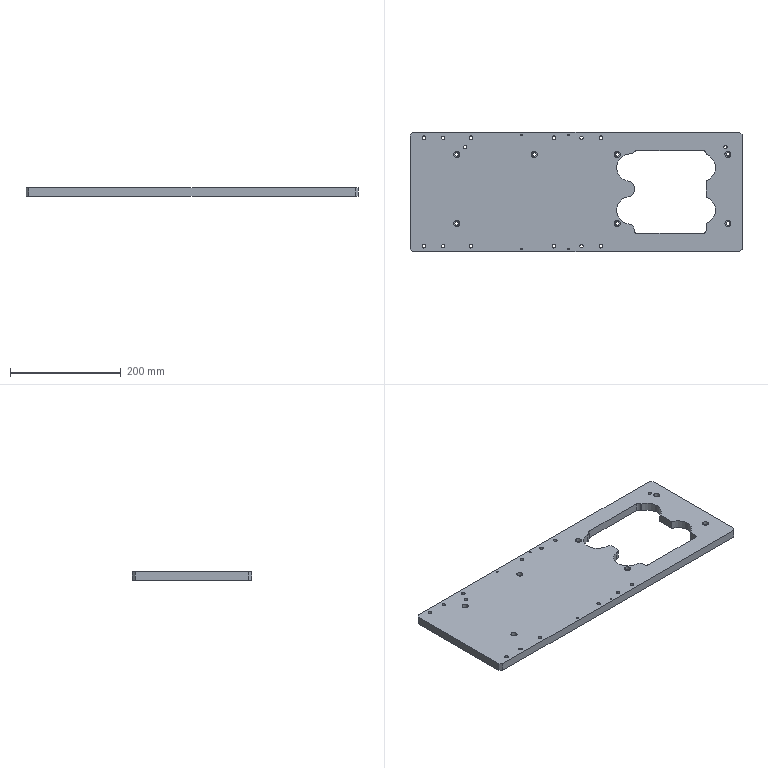Part | 1 solid | 124 faces | box 600 x 216 x 15 mm | volume 1576504 mm3 | cylinder 92 | plane 32 | commonest cylinder face diameters 6.6 x30 11 x30 6 x12 3.3 x8 10 x4 20 x4